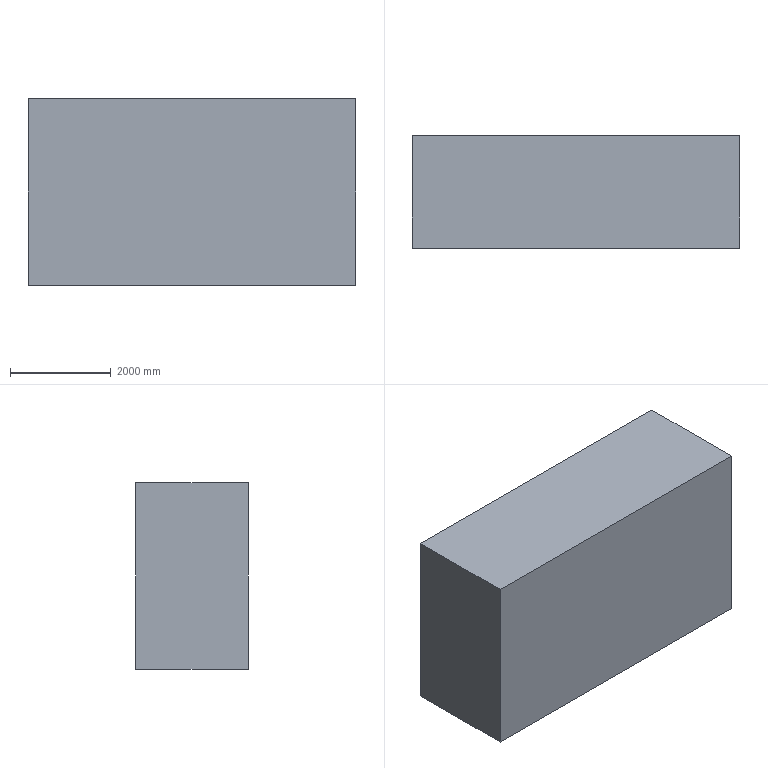Part | SolidWorks | features Extrusion 1, ICE 1 | 1 solid | 12 faces | box 6500 x 2240 x 3710 mm | volume 2774520000 mm3 | plane 12
STEP:
#1=CARTESIAN_POINT('',(3250.,0.,1855.));
#2=VERTEX_POINT('',#1);
#3=CARTESIAN_POINT('',(3250.,0.,-1855.));
#4=VERTEX_POINT('',#3);
#5=CARTESIAN_POINT('',(3250.,0.,-1855.));
#6=DIRECTION('',(0.,0.,-1.));
#7=VECTOR('',#6,1000.);
#8=LINE('',#5,#7);
#9=EDGE_CURVE('',#2,#4,#8,.T.);
#10=ORIENTED_EDGE('',*,*,#9,.T.);
#11=CARTESIAN_POINT('',(3250.,2240.,-1855.));
#12=VERTEX_POINT('',#11);
#13=CARTESIAN_POINT('',(3250.,2240.,-1855.));
#14=DIRECTION('',(0.,-1.,0.));
#15=VECTOR('',#14,1000.);
#16=LINE('',#13,#15);
#17=EDGE_CURVE('',#12,#4,#16,.T.);
#18=ORIENTED_EDGE('',*,*,#17,.F.);
#19=CARTESIAN_POINT('',(3250.,2240.,1855.));
#20=VERTEX_POINT('',#19);
#21=CARTESIAN_POINT('',(3250.,2240.,-1855.));
#22=DIRECTION('',(0.,0.,-1.));
#23=VECTOR('',#22,1000.);
#24=LINE('',#21,#23);
#25=EDGE_CURVE('',#20,#12,#24,.T.);
#26=ORIENTED_EDGE('',*,*,#25,.F.);
#27=CARTESIAN_POINT('',(3250.,2240.,1855.));
#28=DIRECTION('',(0.,-1.,0.));
#29=VECTOR('',#28,1000.);
#30=LINE('',#27,#29);
#31=EDGE_CURVE('',#20,#2,#30,.T.);
#32=ORIENTED_EDGE('',*,*,#31,.T.);
#33=EDGE_LOOP('',(#10,#18,#26,#32));
#34=FACE_OUTER_BOUND('',#33,.T.);
#35=CARTESIAN_POINT('',(3250.,2240.,-1855.));
#36=DIRECTION('',(-1.,0.,0.));
#37=DIRECTION('',(0.,0.,1.));
#38=AXIS2_PLACEMENT_3D('',#35,#36,#37);
#39=PLANE('',#38);
#40=ADVANCED_FACE('',(#34),#39,.F.);
#41=CARTESIAN_POINT('',(-3250.,0.,-1855.));
#42=VERTEX_POINT('',#41);
#43=CARTESIAN_POINT('',(-3250.,0.,-1855.));
#44=DIRECTION('',(-1.,0.,0.));
#45=VECTOR('',#44,1000.);
#46=LINE('',#43,#45);
#47=EDGE_CURVE('',#4,#42,#46,.T.);
#48=ORIENTED_EDGE('',*,*,#47,.T.);
#49=CARTESIAN_POINT('',(-3250.,2240.,-1855.));
#50=VERTEX_POINT('',#49);
#51=CARTESIAN_POINT('',(-3250.,2240.,-1855.));
#52=DIRECTION('',(0.,-1.,0.));
#53=VECTOR('',#52,1000.);
#54=LINE('',#51,#53);
#55=EDGE_CURVE('',#50,#42,#54,.T.);
#56=ORIENTED_EDGE('',*,*,#55,.F.);
#57=CARTESIAN_POINT('',(-3250.,2240.,-1855.));
#58=DIRECTION('',(-1.,0.,0.));
#59=VECTOR('',#58,1000.);
#60=LINE('',#57,#59);
#61=EDGE_CURVE('',#12,#50,#60,.T.);
#62=ORIENTED_EDGE('',*,*,#61,.F.);
#63=ORIENTED_EDGE('',*,*,#17,.T.);
#64=EDGE_LOOP('',(#48,#56,#62,#63));
#65=FACE_OUTER_BOUND('',#64,.T.);
#66=CARTESIAN_POINT('',(-3250.,2240.,-1855.));
#67=DIRECTION('',(0.,0.,1.));
#68=DIRECTION('',(1.,0.,0.));
#69=AXIS2_PLACEMENT_3D('',#66,#67,#68);
#70=PLANE('',#69);
#71=ADVANCED_FACE('',(#65),#70,.F.);
#72=CARTESIAN_POINT('',(-3250.,0.,1855.));
#73=VERTEX_POINT('',#72);
#74=CARTESIAN_POINT('',(-3250.,0.,-1855.));
#75=DIRECTION('',(0.,0.,1.));
#76=VECTOR('',#75,1000.);
#77=LINE('',#74,#76);
#78=EDGE_CURVE('',#42,#73,#77,.T.);
#79=ORIENTED_EDGE('',*,*,#78,.T.);
#80=CARTESIAN_POINT('',(-3250.,2240.,1855.));
#81=VERTEX_POINT('',#80);
#82=CARTESIAN_POINT('',(-3250.,2240.,1855.));
#83=DIRECTION('',(0.,-1.,0.));
#84=VECTOR('',#83,1000.);
#85=LINE('',#82,#84);
#86=EDGE_CURVE('',#81,#73,#85,.T.);
#87=ORIENTED_EDGE('',*,*,#86,.F.);
#88=CARTESIAN_POINT('',(-3250.,2240.,-1855.));
#89=DIRECTION('',(0.,0.,1.));
#90=VECTOR('',#89,1000.);
#91=LINE('',#88,#90);
#92=EDGE_CURVE('',#50,#81,#91,.T.);
#93=ORIENTED_EDGE('',*,*,#92,.F.);
#94=ORIENTED_EDGE('',*,*,#55,.T.);
#95=EDGE_LOOP('',(#79,#87,#93,#94));
#96=FACE_OUTER_BOUND('',#95,.T.);
#97=CARTESIAN_POINT('',(-3250.,2240.,-1855.));
#98=DIRECTION('',(1.,0.,0.));
#99=DIRECTION('',(0.,0.,-1.));
#100=AXIS2_PLACEMENT_3D('',#97,#98,#99);
#101=PLANE('',#100);
#102=ADVANCED_FACE('',(#96),#101,.F.);
#103=CARTESIAN_POINT('',(-3250.,0.,1855.));
#104=DIRECTION('',(1.,0.,0.));
#105=VECTOR('',#104,1000.);
#106=LINE('',#103,#105);
#107=EDGE_CURVE('',#73,#2,#106,.T.);
#108=ORIENTED_EDGE('',*,*,#107,.T.);
#109=ORIENTED_EDGE('',*,*,#31,.F.);
#110=CARTESIAN_POINT('',(-3250.,2240.,1855.));
#111=DIRECTION('',(1.,0.,0.));
#112=VECTOR('',#111,1000.);
#113=LINE('',#110,#112);
#114=EDGE_CURVE('',#81,#20,#113,.T.);
#115=ORIENTED_EDGE('',*,*,#114,.F.);
#116=ORIENTED_EDGE('',*,*,#86,.T.);
#117=EDGE_LOOP('',(#108,#109,#115,#116));
#118=FACE_OUTER_BOUND('',#117,.T.);
#119=CARTESIAN_POINT('',(-3250.,2240.,1855.));
#120=DIRECTION('',(0.,0.,-1.));
#121=DIRECTION('',(-1.,0.,0.));
#122=AXIS2_PLACEMENT_3D('',#119,#120,#121);
#123=PLANE('',#122);
#124=ADVANCED_FACE('',(#118),#123,.F.);
#125=ORIENTED_EDGE('',*,*,#25,.T.);
#126=ORIENTED_EDGE('',*,*,#61,.T.);
#127=ORIENTED_EDGE('',*,*,#92,.T.);
#128=ORIENTED_EDGE('',*,*,#114,.T.);
#129=EDGE_LOOP('',(#125,#126,#127,#128));
#130=FACE_OUTER_BOUND('',#129,.T.);
#131=CARTESIAN_POINT('',(0.,2240.,0.));
#132=DIRECTION('',(0.,1.,0.));
#133=DIRECTION('',(0.,0.,1.));
#134=AXIS2_PLACEMENT_3D('',#131,#132,#133);
#135=PLANE('',#134);
#136=ADVANCED_FACE('',(#130),#135,.T.);
#137=ORIENTED_EDGE('',*,*,#9,.F.);
#138=ORIENTED_EDGE('',*,*,#107,.F.);
#139=ORIENTED_EDGE('',*,*,#78,.F.);
#140=ORIENTED_EDGE('',*,*,#47,.F.);
#141=EDGE_LOOP('',(#137,#138,#139,#140));
#142=FACE_OUTER_BOUND('',#141,.T.);
#143=CARTESIAN_POINT('',(0.,0.,0.));
#144=DIRECTION('',(0.,1.,0.));
#145=DIRECTION('',(0.,0.,1.));
#146=AXIS2_PLACEMENT_3D('',#143,#144,#145);
#147=PLANE('',#146);
#148=ADVANCED_FACE('',(#142),#147,.F.);
#149=CLOSED_SHELL('',(#40,#71,#102,#124,#136,#148));
#150=CARTESIAN_POINT('',(3220.,30.,-1825.));
#151=VERTEX_POINT('',#150);
#152=CARTESIAN_POINT('',(-3220.,30.,-1825.));
#153=VERTEX_POINT('',#152);
#154=CARTESIAN_POINT('',(3220.,30.,-1825.));
#155=DIRECTION('',(-1.,0.,0.));
#156=VECTOR('',#155,1000.);
#157=LINE('',#154,#156);
#158=EDGE_CURVE('',#151,#153,#157,.T.);
#159=ORIENTED_EDGE('',*,*,#158,.F.);
#160=CARTESIAN_POINT('',(3220.,2210.,-1825.));
#161=VERTEX_POINT('',#160);
#162=CARTESIAN_POINT('',(3220.,30.,-1825.));
#163=DIRECTION('',(0.,1.,0.));
#164=VECTOR('',#163,1000.);
#165=LINE('',#162,#164);
#166=EDGE_CURVE('',#151,#161,#165,.T.);
#167=ORIENTED_EDGE('',*,*,#166,.T.);
#168=CARTESIAN_POINT('',(-3220.,2210.,-1825.));
#169=VERTEX_POINT('',#168);
#170=CARTESIAN_POINT('',(3220.,2210.,-1825.));
#171=DIRECTION('',(-1.,0.,0.));
#172=VECTOR('',#171,1000.);
#173=LINE('',#170,#172);
#174=EDGE_CURVE('',#161,#169,#173,.T.);
#175=ORIENTED_EDGE('',*,*,#174,.T.);
#176=CARTESIAN_POINT('',(-3220.,30.,-1825.));
#177=DIRECTION('',(0.,1.,0.));
#178=VECTOR('',#177,1000.);
#179=LINE('',#176,#178);
#180=EDGE_CURVE('',#153,#169,#179,.T.);
#181=ORIENTED_EDGE('',*,*,#180,.F.);
#182=EDGE_LOOP('',(#159,#167,#175,#181));
#183=FACE_OUTER_BOUND('',#182,.T.);
#184=CARTESIAN_POINT('',(3220.,30.,-1825.));
#185=DIRECTION('',(0.,0.,1.));
#186=DIRECTION('',(1.,0.,0.));
#187=AXIS2_PLACEMENT_3D('',#184,#185,#186);
#188=PLANE('',#187);
#189=ADVANCED_FACE('',(#183),#188,.T.);
#190=ORIENTED_EDGE('',*,*,#174,.F.);
#191=CARTESIAN_POINT('',(3220.,2210.,1825.));
#192=VERTEX_POINT('',#191);
#193=CARTESIAN_POINT('',(3220.,2210.,1825.));
#194=DIRECTION('',(0.,0.,1.));
#195=VECTOR('',#194,1000.);
#196=LINE('',#193,#195);
#197=EDGE_CURVE('',#161,#192,#196,.T.);
#198=ORIENTED_EDGE('',*,*,#197,.T.);
#199=CARTESIAN_POINT('',(-3220.,2210.,1825.));
#200=VERTEX_POINT('',#199);
#201=CARTESIAN_POINT('',(3220.,2210.,1825.));
#202=DIRECTION('',(-1.,0.,0.));
#203=VECTOR('',#202,1000.);
#204=LINE('',#201,#203);
#205=EDGE_CURVE('',#192,#200,#204,.T.);
#206=ORIENTED_EDGE('',*,*,#205,.T.);
#207=CARTESIAN_POINT('',(-3220.,2210.,1825.));
#208=DIRECTION('',(0.,0.,1.));
#209=VECTOR('',#208,1000.);
#210=LINE('',#207,#209);
#211=EDGE_CURVE('',#169,#200,#210,.T.);
#212=ORIENTED_EDGE('',*,*,#211,.F.);
#213=EDGE_LOOP('',(#190,#198,#206,#212));
#214=FACE_OUTER_BOUND('',#213,.T.);
#215=CARTESIAN_POINT('',(3220.,2210.,1825.));
#216=DIRECTION('',(0.,-1.,0.));
#217=DIRECTION('',(0.,0.,-1.));
#218=AXIS2_PLACEMENT_3D('',#215,#216,#217);
#219=PLANE('',#218);
#220=ADVANCED_FACE('',(#214),#219,.T.);
#221=ORIENTED_EDGE('',*,*,#205,.F.);
#222=CARTESIAN_POINT('',(3220.,30.,1825.));
#223=VERTEX_POINT('',#222);
#224=CARTESIAN_POINT('',(3220.,30.,1825.));
#225=DIRECTION('',(0.,-1.,0.));
#226=VECTOR('',#225,1000.);
#227=LINE('',#224,#226);
#228=EDGE_CURVE('',#192,#223,#227,.T.);
#229=ORIENTED_EDGE('',*,*,#228,.T.);
#230=CARTESIAN_POINT('',(-3220.,30.,1825.));
#231=VERTEX_POINT('',#230);
#232=CARTESIAN_POINT('',(3220.,30.,1825.));
#233=DIRECTION('',(-1.,0.,0.));
#234=VECTOR('',#233,1000.);
#235=LINE('',#232,#234);
#236=EDGE_CURVE('',#223,#231,#235,.T.);
#237=ORIENTED_EDGE('',*,*,#236,.T.);
#238=CARTESIAN_POINT('',(-3220.,30.,1825.));
#239=DIRECTION('',(0.,-1.,0.));
#240=VECTOR('',#239,1000.);
#241=LINE('',#238,#240);
#242=EDGE_CURVE('',#200,#231,#241,.T.);
#243=ORIENTED_EDGE('',*,*,#242,.F.);
#244=EDGE_LOOP('',(#221,#229,#237,#243));
#245=FACE_OUTER_BOUND('',#244,.T.);
#246=CARTESIAN_POINT('',(3220.,30.,1825.));
#247=DIRECTION('',(0.,0.,-1.));
#248=DIRECTION('',(-1.,0.,0.));
#249=AXIS2_PLACEMENT_3D('',#246,#247,#248);
#250=PLANE('',#249);
#251=ADVANCED_FACE('',(#245),#250,.T.);
#252=ORIENTED_EDGE('',*,*,#236,.F.);
#253=CARTESIAN_POINT('',(3220.,30.,1825.));
#254=DIRECTION('',(0.,0.,-1.));
#255=VECTOR('',#254,1000.);
#256=LINE('',#253,#255);
#257=EDGE_CURVE('',#223,#151,#256,.T.);
#258=ORIENTED_EDGE('',*,*,#257,.T.);
#259=ORIENTED_EDGE('',*,*,#158,.T.);
#260=CARTESIAN_POINT('',(-3220.,30.,1825.));
#261=DIRECTION('',(0.,0.,-1.));
#262=VECTOR('',#261,1000.);
#263=LINE('',#260,#262);
#264=EDGE_CURVE('',#231,#153,#263,.T.);
#265=ORIENTED_EDGE('',*,*,#264,.F.);
#266=EDGE_LOOP('',(#252,#258,#259,#265));
#267=FACE_OUTER_BOUND('',#266,.T.);
#268=CARTESIAN_POINT('',(3220.,30.,1825.));
#269=DIRECTION('',(0.,1.,0.));
#270=DIRECTION('',(0.,0.,1.));
#271=AXIS2_PLACEMENT_3D('',#268,#269,#270);
#272=PLANE('',#271);
#273=ADVANCED_FACE('',(#267),#272,.T.);
#274=ORIENTED_EDGE('',*,*,#166,.F.);
#275=ORIENTED_EDGE('',*,*,#257,.F.);
#276=ORIENTED_EDGE('',*,*,#228,.F.);
#277=ORIENTED_EDGE('',*,*,#197,.F.);
#278=EDGE_LOOP('',(#274,#275,#276,#277));
#279=FACE_OUTER_BOUND('',#278,.T.);
#280=CARTESIAN_POINT('',(3220.,0.,0.));
#281=DIRECTION('',(-1.,0.,0.));
#282=DIRECTION('',(0.,0.,1.));
#283=AXIS2_PLACEMENT_3D('',#280,#281,#282);
#284=PLANE('',#283);
#285=ADVANCED_FACE('',(#279),#284,.T.);
#286=ORIENTED_EDGE('',*,*,#180,.T.);
#287=ORIENTED_EDGE('',*,*,#211,.T.);
#288=ORIENTED_EDGE('',*,*,#242,.T.);
#289=ORIENTED_EDGE('',*,*,#264,.T.);
#290=EDGE_LOOP('',(#286,#287,#288,#289));
#291=FACE_OUTER_BOUND('',#290,.T.);
#292=CARTESIAN_POINT('',(-3220.,0.,0.));
#293=DIRECTION('',(-1.,0.,0.));
#294=DIRECTION('',(0.,0.,1.));
#295=AXIS2_PLACEMENT_3D('',#292,#293,#294);
#296=PLANE('',#295);
#297=ADVANCED_FACE('',(#291),#296,.F.);
#298=CLOSED_SHELL('',(#189,#220,#251,#273,#285,#297));
#299=ORIENTED_CLOSED_SHELL('',*,#298,.F.);
#300=BREP_WITH_VOIDS('',#149,(#299));
#301=CARTESIAN_POINT('',(0.,0.,0.));
#302=DIRECTION('',(0.,0.,1.));
#303=DIRECTION('',(1.,0.,0.));
#304=AXIS2_PLACEMENT_3D('',#301,#302,#303);
#305=(LENGTH_UNIT()NAMED_UNIT(*)SI_UNIT(.MILLI.,.METRE.));
#306=UNCERTAINTY_MEASURE_WITH_UNIT(LENGTH_MEASURE(0.00001),#305,'','');
#307=(NAMED_UNIT(*)PLANE_ANGLE_UNIT()SI_UNIT($,.RADIAN.));
#308=(NAMED_UNIT(*)SI_UNIT($,.STERADIAN.)SOLID_ANGLE_UNIT());
#309=(GEOMETRIC_REPRESENTATION_CONTEXT(3)GLOBAL_UNCERTAINTY_ASSIGNED_CONTEXT((#306))GLOBAL_UNIT_ASSIGNED_CONTEXT((#305,#307,#308))REPRESENTATION_CONTEXT('',''));
#310=ADVANCED_BREP_SHAPE_REPRESENTATION('',(#300,#304),#309);